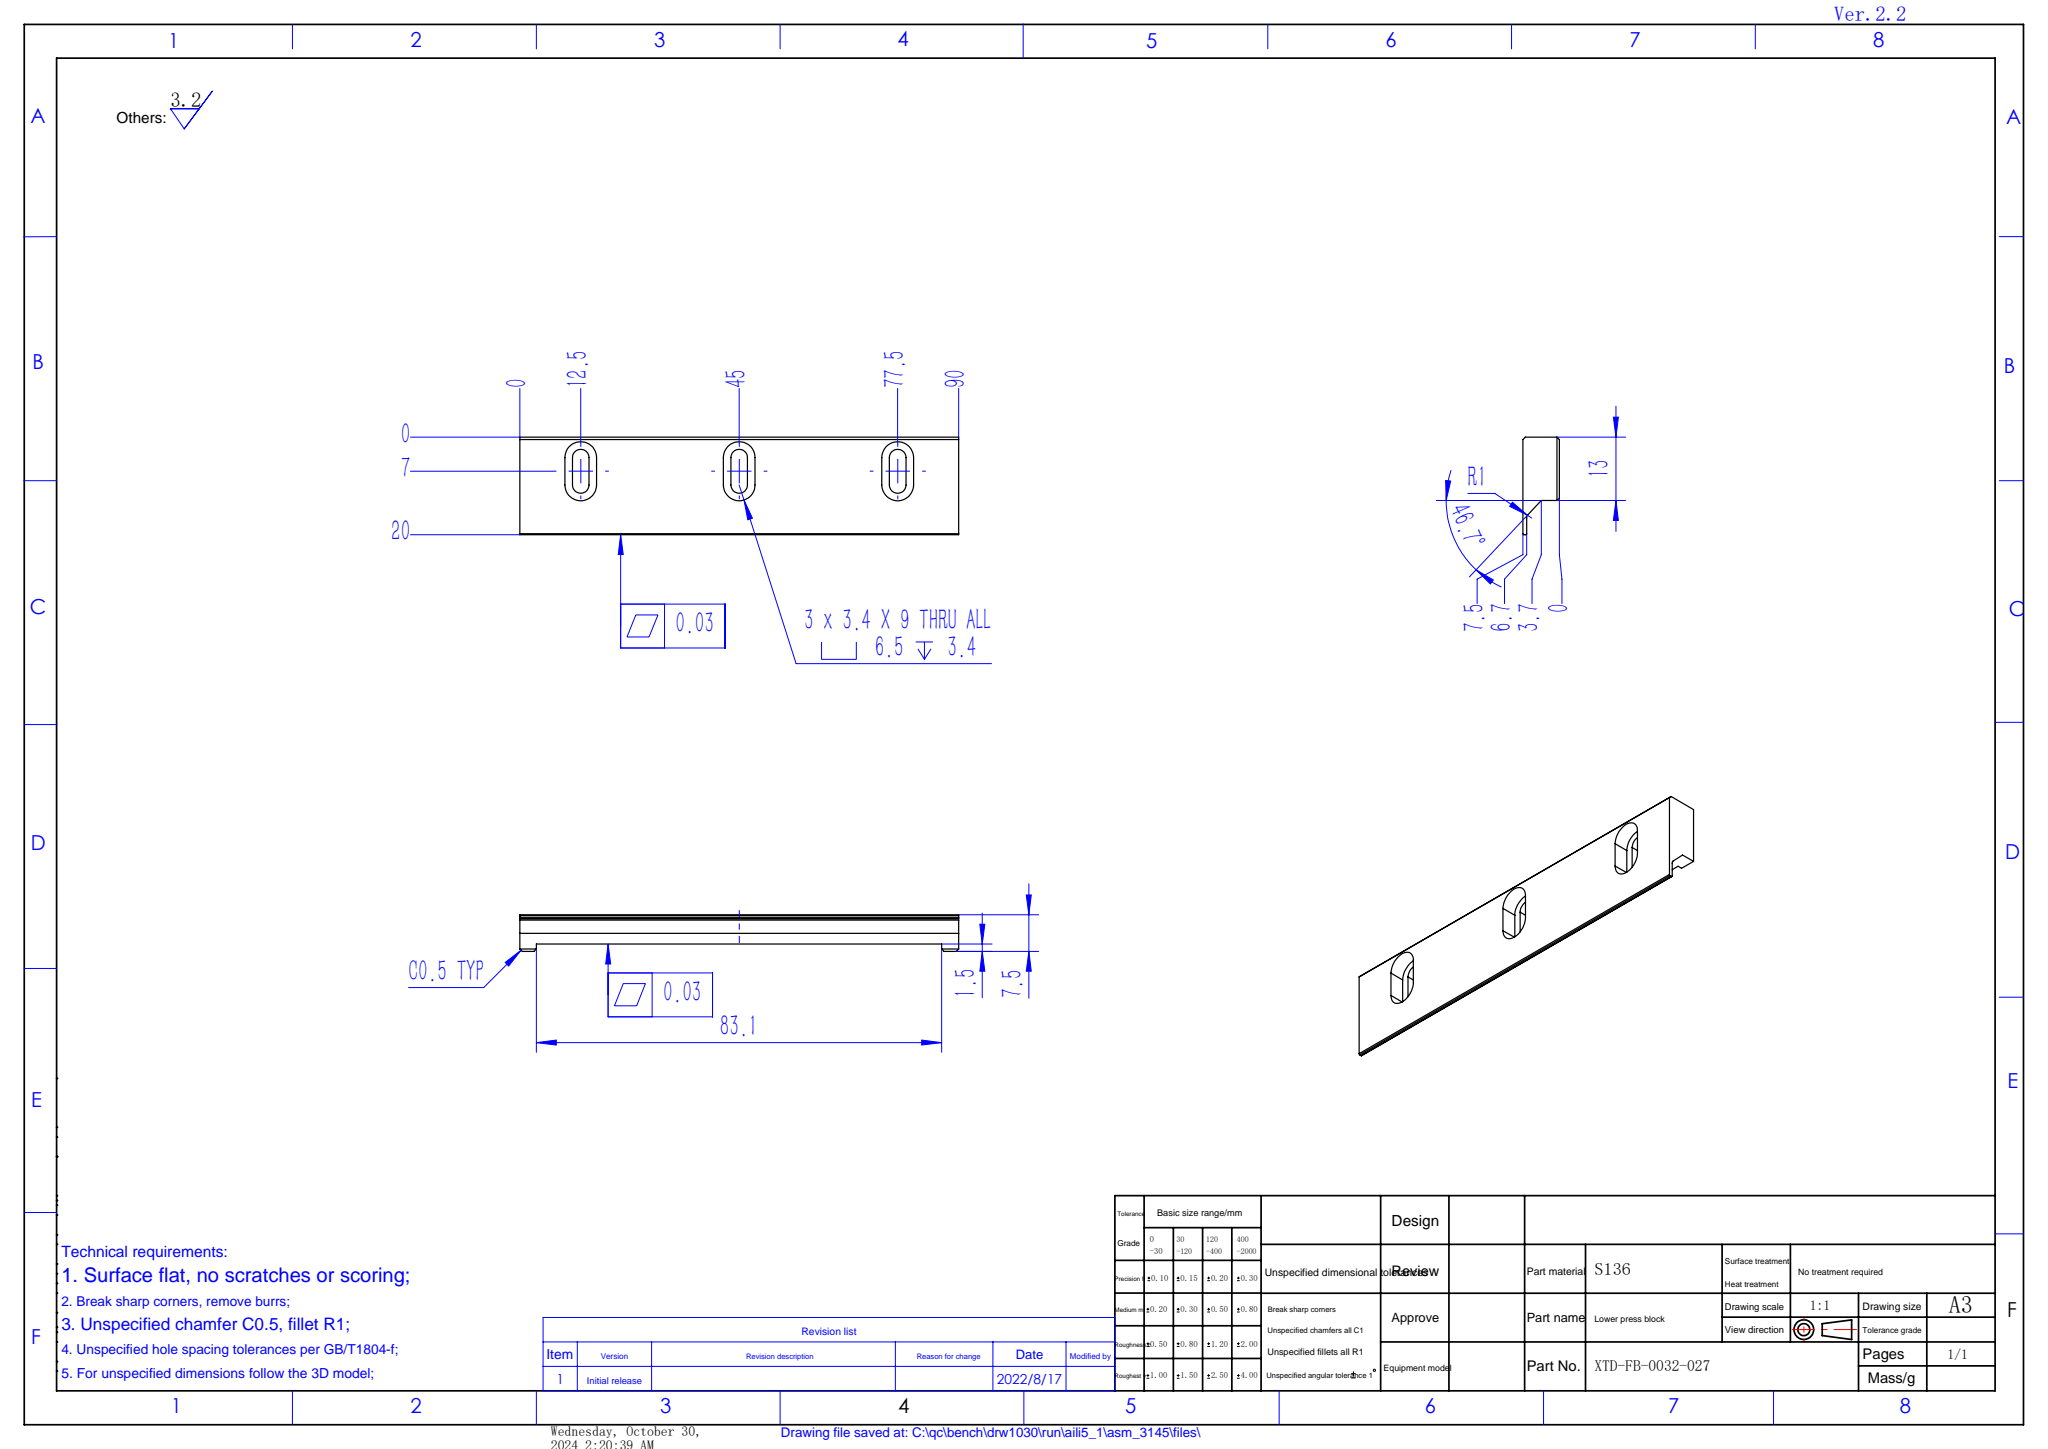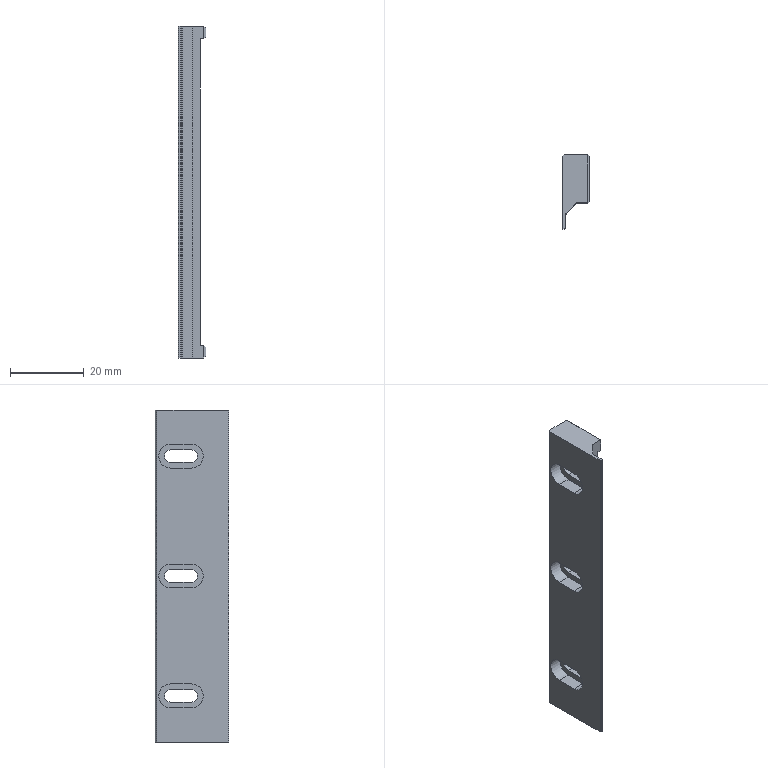Part | SolidWorks | features Chamfer 1, Extrusion 1, Fillet 1, HoleWzd 1, ICE 1 | 1 solid | 52 faces | box 7.5 x 20 x 90 mm | volume 7139 mm3 | plane 37 | cylinder 15 | commonest cylinder face diameters 3.4 x6 6.5 x6 0.4 x2 2 x1